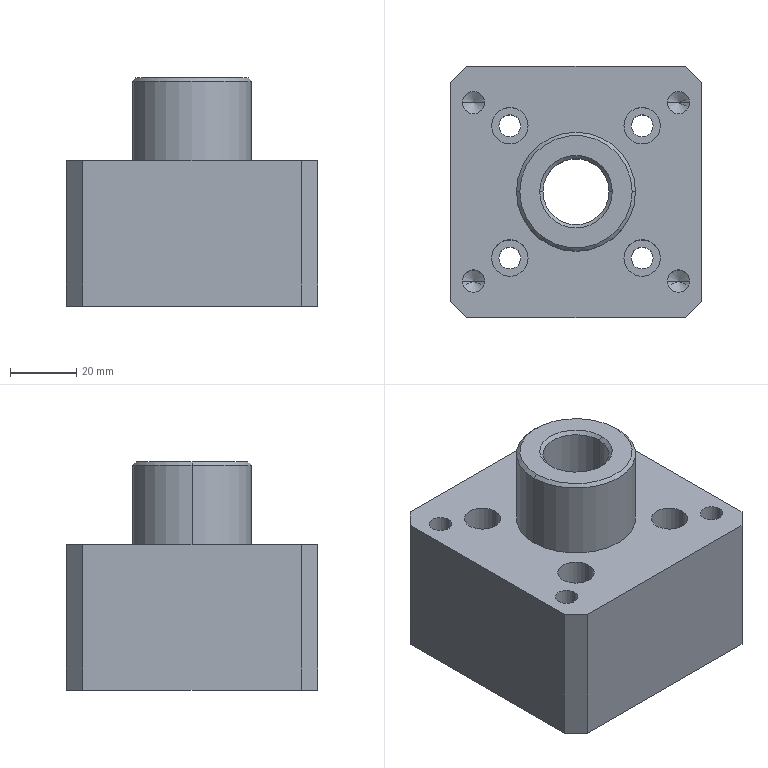Part | STEP file | YCD14007A-08.02.14 Latch Cylinder Seat | 1 solid | 60 faces | box 76 x 76 x 69 mm | volume 233677 mm3 | cylinder 30 | plane 16 | cone 14 | commonest cylinder face diameters 6.6 x8 6.8 x8 11 x8 20 x2 26 x2 36 x2